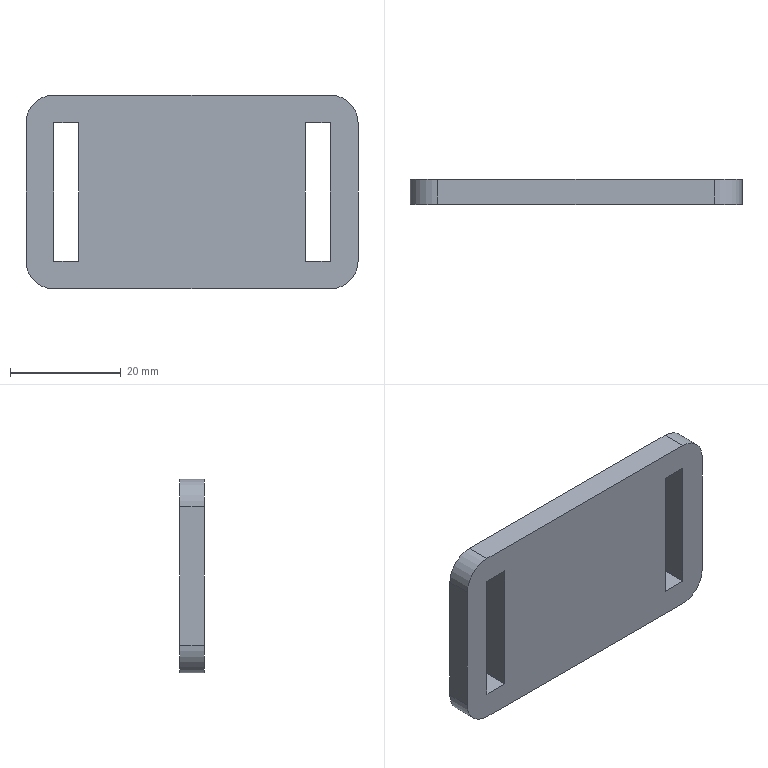Part | SolidWorks | features FlatPattern 1, SMBaseFlange 1, SheetMetal 1 | 1 solid | 18 faces | box 60 x 4.5 x 35 mm | volume 8341 mm3 | plane 14 | cylinder 4 | commonest cylinder face diameters 10 x4
STEP:
#1=CARTESIAN_POINT('',(-30.,0.,12.5));
#2=VERTEX_POINT('',#1);
#3=CARTESIAN_POINT('',(-25.,0.,17.5));
#4=VERTEX_POINT('',#3);
#5=CARTESIAN_POINT('',(-25.,0.,12.5));
#6=DIRECTION('',(0.,1.,0.));
#7=DIRECTION('',(0.,0.,1.));
#8=AXIS2_PLACEMENT_3D('',#5,#6,#7);
#9=CIRCLE('',#8,5.);
#10=EDGE_CURVE('',#2,#4,#9,.T.);
#11=ORIENTED_EDGE('',*,*,#10,.F.);
#12=CARTESIAN_POINT('',(-30.,-4.5,12.5));
#13=VERTEX_POINT('',#12);
#14=CARTESIAN_POINT('',(-30.,-4.5,12.5));
#15=DIRECTION('',(0.,1.,0.));
#16=VECTOR('',#15,1000.);
#17=LINE('',#14,#16);
#18=EDGE_CURVE('',#13,#2,#17,.T.);
#19=ORIENTED_EDGE('',*,*,#18,.F.);
#20=CARTESIAN_POINT('',(-25.,-4.5,17.5));
#21=VERTEX_POINT('',#20);
#22=CARTESIAN_POINT('',(-25.,-4.5,12.5));
#23=DIRECTION('',(0.,1.,0.));
#24=DIRECTION('',(0.,0.,1.));
#25=AXIS2_PLACEMENT_3D('',#22,#23,#24);
#26=CIRCLE('',#25,5.);
#27=EDGE_CURVE('',#13,#21,#26,.T.);
#28=ORIENTED_EDGE('',*,*,#27,.T.);
#29=CARTESIAN_POINT('',(-25.,-4.5,17.5));
#30=DIRECTION('',(0.,1.,0.));
#31=VECTOR('',#30,1000.);
#32=LINE('',#29,#31);
#33=EDGE_CURVE('',#21,#4,#32,.T.);
#34=ORIENTED_EDGE('',*,*,#33,.T.);
#35=EDGE_LOOP('',(#11,#19,#28,#34));
#36=FACE_OUTER_BOUND('',#35,.T.);
#37=CARTESIAN_POINT('',(-25.,-4.5,12.5));
#38=DIRECTION('',(0.,1.,0.));
#39=DIRECTION('',(0.,0.,1.));
#40=AXIS2_PLACEMENT_3D('',#37,#38,#39);
#41=CYLINDRICAL_SURFACE('',#40,5.);
#42=ADVANCED_FACE('',(#36),#41,.T.);
#43=CARTESIAN_POINT('',(-30.,0.,-12.5));
#44=VERTEX_POINT('',#43);
#45=CARTESIAN_POINT('',(-30.,0.,-12.5));
#46=DIRECTION('',(0.,0.,1.));
#47=VECTOR('',#46,1000.);
#48=LINE('',#45,#47);
#49=EDGE_CURVE('',#44,#2,#48,.T.);
#50=ORIENTED_EDGE('',*,*,#49,.F.);
#51=CARTESIAN_POINT('',(-30.,-4.5,-12.5));
#52=VERTEX_POINT('',#51);
#53=CARTESIAN_POINT('',(-30.,-4.5,-12.5));
#54=DIRECTION('',(0.,1.,0.));
#55=VECTOR('',#54,1000.);
#56=LINE('',#53,#55);
#57=EDGE_CURVE('',#52,#44,#56,.T.);
#58=ORIENTED_EDGE('',*,*,#57,.F.);
#59=CARTESIAN_POINT('',(-30.,-4.5,-12.5));
#60=DIRECTION('',(0.,0.,1.));
#61=VECTOR('',#60,1000.);
#62=LINE('',#59,#61);
#63=EDGE_CURVE('',#52,#13,#62,.T.);
#64=ORIENTED_EDGE('',*,*,#63,.T.);
#65=ORIENTED_EDGE('',*,*,#18,.T.);
#66=EDGE_LOOP('',(#50,#58,#64,#65));
#67=FACE_OUTER_BOUND('',#66,.T.);
#68=CARTESIAN_POINT('',(-30.,-4.5,-12.5));
#69=DIRECTION('',(-1.,0.,0.));
#70=DIRECTION('',(0.,0.,1.));
#71=AXIS2_PLACEMENT_3D('',#68,#69,#70);
#72=PLANE('',#71);
#73=ADVANCED_FACE('',(#67),#72,.T.);
#74=CARTESIAN_POINT('',(-25.,0.,-17.5));
#75=VERTEX_POINT('',#74);
#76=CARTESIAN_POINT('',(-25.,0.,-12.5));
#77=DIRECTION('',(0.,1.,0.));
#78=DIRECTION('',(0.,0.,1.));
#79=AXIS2_PLACEMENT_3D('',#76,#77,#78);
#80=CIRCLE('',#79,5.);
#81=EDGE_CURVE('',#75,#44,#80,.T.);
#82=ORIENTED_EDGE('',*,*,#81,.F.);
#83=CARTESIAN_POINT('',(-25.,-4.5,-17.5));
#84=VERTEX_POINT('',#83);
#85=CARTESIAN_POINT('',(-25.,-4.5,-17.5));
#86=DIRECTION('',(0.,1.,0.));
#87=VECTOR('',#86,1000.);
#88=LINE('',#85,#87);
#89=EDGE_CURVE('',#84,#75,#88,.T.);
#90=ORIENTED_EDGE('',*,*,#89,.F.);
#91=CARTESIAN_POINT('',(-25.,-4.5,-12.5));
#92=DIRECTION('',(0.,1.,0.));
#93=DIRECTION('',(0.,0.,1.));
#94=AXIS2_PLACEMENT_3D('',#91,#92,#93);
#95=CIRCLE('',#94,5.);
#96=EDGE_CURVE('',#84,#52,#95,.T.);
#97=ORIENTED_EDGE('',*,*,#96,.T.);
#98=ORIENTED_EDGE('',*,*,#57,.T.);
#99=EDGE_LOOP('',(#82,#90,#97,#98));
#100=FACE_OUTER_BOUND('',#99,.T.);
#101=CARTESIAN_POINT('',(-25.,-4.5,-12.5));
#102=DIRECTION('',(0.,1.,0.));
#103=DIRECTION('',(0.,0.,1.));
#104=AXIS2_PLACEMENT_3D('',#101,#102,#103);
#105=CYLINDRICAL_SURFACE('',#104,5.);
#106=ADVANCED_FACE('',(#100),#105,.T.);
#107=CARTESIAN_POINT('',(25.,0.,-17.5));
#108=VERTEX_POINT('',#107);
#109=CARTESIAN_POINT('',(-25.,0.,-17.5));
#110=DIRECTION('',(-1.,0.,0.));
#111=VECTOR('',#110,1000.);
#112=LINE('',#109,#111);
#113=EDGE_CURVE('',#108,#75,#112,.T.);
#114=ORIENTED_EDGE('',*,*,#113,.F.);
#115=CARTESIAN_POINT('',(25.,-4.5,-17.5));
#116=VERTEX_POINT('',#115);
#117=CARTESIAN_POINT('',(25.,-4.5,-17.5));
#118=DIRECTION('',(0.,1.,0.));
#119=VECTOR('',#118,1000.);
#120=LINE('',#117,#119);
#121=EDGE_CURVE('',#116,#108,#120,.T.);
#122=ORIENTED_EDGE('',*,*,#121,.F.);
#123=CARTESIAN_POINT('',(-25.,-4.5,-17.5));
#124=DIRECTION('',(-1.,0.,0.));
#125=VECTOR('',#124,1000.);
#126=LINE('',#123,#125);
#127=EDGE_CURVE('',#116,#84,#126,.T.);
#128=ORIENTED_EDGE('',*,*,#127,.T.);
#129=ORIENTED_EDGE('',*,*,#89,.T.);
#130=EDGE_LOOP('',(#114,#122,#128,#129));
#131=FACE_OUTER_BOUND('',#130,.T.);
#132=CARTESIAN_POINT('',(-25.,-4.5,-17.5));
#133=DIRECTION('',(0.,0.,-1.));
#134=DIRECTION('',(-1.,0.,0.));
#135=AXIS2_PLACEMENT_3D('',#132,#133,#134);
#136=PLANE('',#135);
#137=ADVANCED_FACE('',(#131),#136,.T.);
#138=CARTESIAN_POINT('',(30.,0.,-12.5));
#139=VERTEX_POINT('',#138);
#140=CARTESIAN_POINT('',(25.,0.,-12.5));
#141=DIRECTION('',(0.,1.,0.));
#142=DIRECTION('',(0.,0.,-1.));
#143=AXIS2_PLACEMENT_3D('',#140,#141,#142);
#144=CIRCLE('',#143,5.);
#145=EDGE_CURVE('',#139,#108,#144,.T.);
#146=ORIENTED_EDGE('',*,*,#145,.F.);
#147=CARTESIAN_POINT('',(30.,-4.5,-12.5));
#148=VERTEX_POINT('',#147);
#149=CARTESIAN_POINT('',(30.,-4.5,-12.5));
#150=DIRECTION('',(0.,1.,0.));
#151=VECTOR('',#150,1000.);
#152=LINE('',#149,#151);
#153=EDGE_CURVE('',#148,#139,#152,.T.);
#154=ORIENTED_EDGE('',*,*,#153,.F.);
#155=CARTESIAN_POINT('',(25.,-4.5,-12.5));
#156=DIRECTION('',(0.,1.,0.));
#157=DIRECTION('',(0.,0.,-1.));
#158=AXIS2_PLACEMENT_3D('',#155,#156,#157);
#159=CIRCLE('',#158,5.);
#160=EDGE_CURVE('',#148,#116,#159,.T.);
#161=ORIENTED_EDGE('',*,*,#160,.T.);
#162=ORIENTED_EDGE('',*,*,#121,.T.);
#163=EDGE_LOOP('',(#146,#154,#161,#162));
#164=FACE_OUTER_BOUND('',#163,.T.);
#165=CARTESIAN_POINT('',(25.,-4.5,-12.5));
#166=DIRECTION('',(0.,1.,0.));
#167=DIRECTION('',(0.,0.,1.));
#168=AXIS2_PLACEMENT_3D('',#165,#166,#167);
#169=CYLINDRICAL_SURFACE('',#168,5.);
#170=ADVANCED_FACE('',(#164),#169,.T.);
#171=CARTESIAN_POINT('',(30.,0.,12.5));
#172=VERTEX_POINT('',#171);
#173=CARTESIAN_POINT('',(30.,0.,-12.5));
#174=DIRECTION('',(0.,0.,-1.));
#175=VECTOR('',#174,1000.);
#176=LINE('',#173,#175);
#177=EDGE_CURVE('',#172,#139,#176,.T.);
#178=ORIENTED_EDGE('',*,*,#177,.F.);
#179=CARTESIAN_POINT('',(30.,-4.5,12.5));
#180=VERTEX_POINT('',#179);
#181=CARTESIAN_POINT('',(30.,-4.5,12.5));
#182=DIRECTION('',(0.,1.,0.));
#183=VECTOR('',#182,1000.);
#184=LINE('',#181,#183);
#185=EDGE_CURVE('',#180,#172,#184,.T.);
#186=ORIENTED_EDGE('',*,*,#185,.F.);
#187=CARTESIAN_POINT('',(30.,-4.5,-12.5));
#188=DIRECTION('',(0.,0.,-1.));
#189=VECTOR('',#188,1000.);
#190=LINE('',#187,#189);
#191=EDGE_CURVE('',#180,#148,#190,.T.);
#192=ORIENTED_EDGE('',*,*,#191,.T.);
#193=ORIENTED_EDGE('',*,*,#153,.T.);
#194=EDGE_LOOP('',(#178,#186,#192,#193));
#195=FACE_OUTER_BOUND('',#194,.T.);
#196=CARTESIAN_POINT('',(30.,-4.5,-12.5));
#197=DIRECTION('',(1.,0.,0.));
#198=DIRECTION('',(0.,0.,-1.));
#199=AXIS2_PLACEMENT_3D('',#196,#197,#198);
#200=PLANE('',#199);
#201=ADVANCED_FACE('',(#195),#200,.T.);
#202=CARTESIAN_POINT('',(25.,0.,17.5));
#203=VERTEX_POINT('',#202);
#204=CARTESIAN_POINT('',(25.,0.,12.5));
#205=DIRECTION('',(0.,1.,0.));
#206=DIRECTION('',(0.,0.,1.));
#207=AXIS2_PLACEMENT_3D('',#204,#205,#206);
#208=CIRCLE('',#207,5.);
#209=EDGE_CURVE('',#203,#172,#208,.T.);
#210=ORIENTED_EDGE('',*,*,#209,.F.);
#211=CARTESIAN_POINT('',(25.,-4.5,17.5));
#212=VERTEX_POINT('',#211);
#213=CARTESIAN_POINT('',(25.,-4.5,17.5));
#214=DIRECTION('',(0.,1.,0.));
#215=VECTOR('',#214,1000.);
#216=LINE('',#213,#215);
#217=EDGE_CURVE('',#212,#203,#216,.T.);
#218=ORIENTED_EDGE('',*,*,#217,.F.);
#219=CARTESIAN_POINT('',(25.,-4.5,12.5));
#220=DIRECTION('',(0.,1.,0.));
#221=DIRECTION('',(0.,0.,1.));
#222=AXIS2_PLACEMENT_3D('',#219,#220,#221);
#223=CIRCLE('',#222,5.);
#224=EDGE_CURVE('',#212,#180,#223,.T.);
#225=ORIENTED_EDGE('',*,*,#224,.T.);
#226=ORIENTED_EDGE('',*,*,#185,.T.);
#227=EDGE_LOOP('',(#210,#218,#225,#226));
#228=FACE_OUTER_BOUND('',#227,.T.);
#229=CARTESIAN_POINT('',(25.,-4.5,12.5));
#230=DIRECTION('',(0.,1.,0.));
#231=DIRECTION('',(0.,0.,1.));
#232=AXIS2_PLACEMENT_3D('',#229,#230,#231);
#233=CYLINDRICAL_SURFACE('',#232,5.);
#234=ADVANCED_FACE('',(#228),#233,.T.);
#235=CARTESIAN_POINT('',(-25.,0.,17.5));
#236=DIRECTION('',(1.,0.,0.));
#237=VECTOR('',#236,1000.);
#238=LINE('',#235,#237);
#239=EDGE_CURVE('',#4,#203,#238,.T.);
#240=ORIENTED_EDGE('',*,*,#239,.F.);
#241=ORIENTED_EDGE('',*,*,#33,.F.);
#242=CARTESIAN_POINT('',(-25.,-4.5,17.5));
#243=DIRECTION('',(1.,0.,0.));
#244=VECTOR('',#243,1000.);
#245=LINE('',#242,#244);
#246=EDGE_CURVE('',#21,#212,#245,.T.);
#247=ORIENTED_EDGE('',*,*,#246,.T.);
#248=ORIENTED_EDGE('',*,*,#217,.T.);
#249=EDGE_LOOP('',(#240,#241,#247,#248));
#250=FACE_OUTER_BOUND('',#249,.T.);
#251=CARTESIAN_POINT('',(-25.,-4.5,17.5));
#252=DIRECTION('',(0.,0.,1.));
#253=DIRECTION('',(1.,0.,0.));
#254=AXIS2_PLACEMENT_3D('',#251,#252,#253);
#255=PLANE('',#254);
#256=ADVANCED_FACE('',(#250),#255,.T.);
#257=CARTESIAN_POINT('',(25.,-4.5,12.5));
#258=VERTEX_POINT('',#257);
#259=CARTESIAN_POINT('',(25.,-4.5,-12.5));
#260=VERTEX_POINT('',#259);
#261=CARTESIAN_POINT('',(25.,-4.5,-12.5));
#262=DIRECTION('',(0.,0.,-1.));
#263=VECTOR('',#262,1000.);
#264=LINE('',#261,#263);
#265=EDGE_CURVE('',#258,#260,#264,.T.);
#266=ORIENTED_EDGE('',*,*,#265,.T.);
#267=CARTESIAN_POINT('',(20.5,-4.5,-12.5));
#268=VERTEX_POINT('',#267);
#269=CARTESIAN_POINT('',(25.,-4.5,-12.5));
#270=DIRECTION('',(-1.,0.,0.));
#271=VECTOR('',#270,1000.);
#272=LINE('',#269,#271);
#273=EDGE_CURVE('',#260,#268,#272,.T.);
#274=ORIENTED_EDGE('',*,*,#273,.T.);
#275=CARTESIAN_POINT('',(20.5,-4.5,12.5));
#276=VERTEX_POINT('',#275);
#277=CARTESIAN_POINT('',(20.5,-4.5,-12.5));
#278=DIRECTION('',(0.,0.,1.));
#279=VECTOR('',#278,1000.);
#280=LINE('',#277,#279);
#281=EDGE_CURVE('',#268,#276,#280,.T.);
#282=ORIENTED_EDGE('',*,*,#281,.T.);
#283=CARTESIAN_POINT('',(25.,-4.5,12.5));
#284=DIRECTION('',(1.,0.,0.));
#285=VECTOR('',#284,1000.);
#286=LINE('',#283,#285);
#287=EDGE_CURVE('',#276,#258,#286,.T.);
#288=ORIENTED_EDGE('',*,*,#287,.T.);
#289=EDGE_LOOP('',(#266,#274,#282,#288));
#290=FACE_BOUND('',#289,.T.);
#291=CARTESIAN_POINT('',(-20.5,-4.5,-12.5));
#292=VERTEX_POINT('',#291);
#293=CARTESIAN_POINT('',(-25.,-4.5,-12.5));
#294=VERTEX_POINT('',#293);
#295=CARTESIAN_POINT('',(-25.,-4.5,-12.5));
#296=DIRECTION('',(-1.,0.,0.));
#297=VECTOR('',#296,1000.);
#298=LINE('',#295,#297);
#299=EDGE_CURVE('',#292,#294,#298,.T.);
#300=ORIENTED_EDGE('',*,*,#299,.T.);
#301=CARTESIAN_POINT('',(-25.,-4.5,12.5));
#302=VERTEX_POINT('',#301);
#303=CARTESIAN_POINT('',(-25.,-4.5,-12.5));
#304=DIRECTION('',(0.,0.,1.));
#305=VECTOR('',#304,1000.);
#306=LINE('',#303,#305);
#307=EDGE_CURVE('',#294,#302,#306,.T.);
#308=ORIENTED_EDGE('',*,*,#307,.T.);
#309=CARTESIAN_POINT('',(-20.5,-4.5,12.5));
#310=VERTEX_POINT('',#309);
#311=CARTESIAN_POINT('',(-25.,-4.5,12.5));
#312=DIRECTION('',(1.,0.,0.));
#313=VECTOR('',#312,1000.);
#314=LINE('',#311,#313);
#315=EDGE_CURVE('',#302,#310,#314,.T.);
#316=ORIENTED_EDGE('',*,*,#315,.T.);
#317=CARTESIAN_POINT('',(-20.5,-4.5,-12.5));
#318=DIRECTION('',(0.,0.,-1.));
#319=VECTOR('',#318,1000.);
#320=LINE('',#317,#319);
#321=EDGE_CURVE('',#310,#292,#320,.T.);
#322=ORIENTED_EDGE('',*,*,#321,.T.);
#323=EDGE_LOOP('',(#300,#308,#316,#322));
#324=FACE_BOUND('',#323,.T.);
#325=ORIENTED_EDGE('',*,*,#27,.F.);
#326=ORIENTED_EDGE('',*,*,#63,.F.);
#327=ORIENTED_EDGE('',*,*,#96,.F.);
#328=ORIENTED_EDGE('',*,*,#127,.F.);
#329=ORIENTED_EDGE('',*,*,#160,.F.);
#330=ORIENTED_EDGE('',*,*,#191,.F.);
#331=ORIENTED_EDGE('',*,*,#224,.F.);
#332=ORIENTED_EDGE('',*,*,#246,.F.);
#333=EDGE_LOOP('',(#325,#326,#327,#328,#329,#330,#331,#332));
#334=FACE_OUTER_BOUND('',#333,.T.);
#335=CARTESIAN_POINT('',(-25.,-4.5,12.5));
#336=DIRECTION('',(0.,1.,0.));
#337=DIRECTION('',(0.,0.,1.));
#338=AXIS2_PLACEMENT_3D('',#335,#336,#337);
#339=PLANE('',#338);
#340=ADVANCED_FACE('',(#290,#324,#334),#339,.F.);
#341=CARTESIAN_POINT('',(25.,0.,-12.5));
#342=VERTEX_POINT('',#341);
#343=CARTESIAN_POINT('',(20.5,0.,-12.5));
#344=VERTEX_POINT('',#343);
#345=CARTESIAN_POINT('',(25.,0.,-12.5));
#346=DIRECTION('',(-1.,0.,0.));
#347=VECTOR('',#346,1000.);
#348=LINE('',#345,#347);
#349=EDGE_CURVE('',#342,#344,#348,.T.);
#350=ORIENTED_EDGE('',*,*,#349,.F.);
#351=CARTESIAN_POINT('',(25.,0.,12.5));
#352=VERTEX_POINT('',#351);
#353=CARTESIAN_POINT('',(25.,0.,-12.5));
#354=DIRECTION('',(0.,0.,-1.));
#355=VECTOR('',#354,1000.);
#356=LINE('',#353,#355);
#357=EDGE_CURVE('',#352,#342,#356,.T.);
#358=ORIENTED_EDGE('',*,*,#357,.F.);
#359=CARTESIAN_POINT('',(20.5,0.,12.5));
#360=VERTEX_POINT('',#359);
#361=CARTESIAN_POINT('',(25.,0.,12.5));
#362=DIRECTION('',(1.,0.,0.));
#363=VECTOR('',#362,1000.);
#364=LINE('',#361,#363);
#365=EDGE_CURVE('',#360,#352,#364,.T.);
#366=ORIENTED_EDGE('',*,*,#365,.F.);
#367=CARTESIAN_POINT('',(20.5,0.,-12.5));
#368=DIRECTION('',(0.,0.,1.));
#369=VECTOR('',#368,1000.);
#370=LINE('',#367,#369);
#371=EDGE_CURVE('',#344,#360,#370,.T.);
#372=ORIENTED_EDGE('',*,*,#371,.F.);
#373=EDGE_LOOP('',(#350,#358,#366,#372));
#374=FACE_BOUND('',#373,.T.);
#375=CARTESIAN_POINT('',(-25.,0.,-12.5));
#376=VERTEX_POINT('',#375);
#377=CARTESIAN_POINT('',(-25.,0.,12.5));
#378=VERTEX_POINT('',#377);
#379=CARTESIAN_POINT('',(-25.,0.,-12.5));
#380=DIRECTION('',(0.,0.,1.));
#381=VECTOR('',#380,1000.);
#382=LINE('',#379,#381);
#383=EDGE_CURVE('',#376,#378,#382,.T.);
#384=ORIENTED_EDGE('',*,*,#383,.F.);
#385=CARTESIAN_POINT('',(-20.5,0.,-12.5));
#386=VERTEX_POINT('',#385);
#387=CARTESIAN_POINT('',(-25.,0.,-12.5));
#388=DIRECTION('',(-1.,0.,0.));
#389=VECTOR('',#388,1000.);
#390=LINE('',#387,#389);
#391=EDGE_CURVE('',#386,#376,#390,.T.);
#392=ORIENTED_EDGE('',*,*,#391,.F.);
#393=CARTESIAN_POINT('',(-20.5,0.,12.5));
#394=VERTEX_POINT('',#393);
#395=CARTESIAN_POINT('',(-20.5,0.,-12.5));
#396=DIRECTION('',(0.,0.,-1.));
#397=VECTOR('',#396,1000.);
#398=LINE('',#395,#397);
#399=EDGE_CURVE('',#394,#386,#398,.T.);
#400=ORIENTED_EDGE('',*,*,#399,.F.);
#401=CARTESIAN_POINT('',(-25.,0.,12.5));
#402=DIRECTION('',(1.,0.,0.));
#403=VECTOR('',#402,1000.);
#404=LINE('',#401,#403);
#405=EDGE_CURVE('',#378,#394,#404,.T.);
#406=ORIENTED_EDGE('',*,*,#405,.F.);
#407=EDGE_LOOP('',(#384,#392,#400,#406));
#408=FACE_BOUND('',#407,.T.);
#409=ORIENTED_EDGE('',*,*,#10,.T.);
#410=ORIENTED_EDGE('',*,*,#239,.T.);
#411=ORIENTED_EDGE('',*,*,#209,.T.);
#412=ORIENTED_EDGE('',*,*,#177,.T.);
#413=ORIENTED_EDGE('',*,*,#145,.T.);
#414=ORIENTED_EDGE('',*,*,#113,.T.);
#415=ORIENTED_EDGE('',*,*,#81,.T.);
#416=ORIENTED_EDGE('',*,*,#49,.T.);
#417=EDGE_LOOP('',(#409,#410,#411,#412,#413,#414,#415,#416));
#418=FACE_OUTER_BOUND('',#417,.T.);
#419=CARTESIAN_POINT('',(-25.,0.,12.5));
#420=DIRECTION('',(0.,1.,0.));
#421=DIRECTION('',(0.,0.,1.));
#422=AXIS2_PLACEMENT_3D('',#419,#420,#421);
#423=PLANE('',#422);
#424=ADVANCED_FACE('',(#374,#408,#418),#423,.T.);
#425=ORIENTED_EDGE('',*,*,#383,.T.);
#426=CARTESIAN_POINT('',(-25.,-4.5,12.5));
#427=DIRECTION('',(0.,1.,0.));
#428=VECTOR('',#427,1000.);
#429=LINE('',#426,#428);
#430=EDGE_CURVE('',#302,#378,#429,.T.);
#431=ORIENTED_EDGE('',*,*,#430,.F.);
#432=ORIENTED_EDGE('',*,*,#307,.F.);
#433=CARTESIAN_POINT('',(-25.,-4.5,-12.5));
#434=DIRECTION('',(0.,1.,0.));
#435=VECTOR('',#434,1000.);
#436=LINE('',#433,#435);
#437=EDGE_CURVE('',#294,#376,#436,.T.);
#438=ORIENTED_EDGE('',*,*,#437,.T.);
#439=EDGE_LOOP('',(#425,#431,#432,#438));
#440=FACE_OUTER_BOUND('',#439,.T.);
#441=CARTESIAN_POINT('',(-25.,-4.5,-12.5));
#442=DIRECTION('',(-1.,0.,0.));
#443=DIRECTION('',(0.,0.,1.));
#444=AXIS2_PLACEMENT_3D('',#441,#442,#443);
#445=PLANE('',#444);
#446=ADVANCED_FACE('',(#440),#445,.F.);
#447=ORIENTED_EDGE('',*,*,#391,.T.);
#448=ORIENTED_EDGE('',*,*,#437,.F.);
#449=ORIENTED_EDGE('',*,*,#299,.F.);
#450=CARTESIAN_POINT('',(-20.5,-4.5,-12.5));
#451=DIRECTION('',(0.,1.,0.));
#452=VECTOR('',#451,1000.);
#453=LINE('',#450,#452);
#454=EDGE_CURVE('',#292,#386,#453,.T.);
#455=ORIENTED_EDGE('',*,*,#454,.T.);
#456=EDGE_LOOP('',(#447,#448,#449,#455));
#457=FACE_OUTER_BOUND('',#456,.T.);
#458=CARTESIAN_POINT('',(-25.,-4.5,-12.5));
#459=DIRECTION('',(0.,0.,-1.));
#460=DIRECTION('',(-1.,0.,0.));
#461=AXIS2_PLACEMENT_3D('',#458,#459,#460);
#462=PLANE('',#461);
#463=ADVANCED_FACE('',(#457),#462,.F.);
#464=ORIENTED_EDGE('',*,*,#399,.T.);
#465=ORIENTED_EDGE('',*,*,#454,.F.);
#466=ORIENTED_EDGE('',*,*,#321,.F.);
#467=CARTESIAN_POINT('',(-20.5,-4.5,12.5));
#468=DIRECTION('',(0.,1.,0.));
#469=VECTOR('',#468,1000.);
#470=LINE('',#467,#469);
#471=EDGE_CURVE('',#310,#394,#470,.T.);
#472=ORIENTED_EDGE('',*,*,#471,.T.);
#473=EDGE_LOOP('',(#464,#465,#466,#472));
#474=FACE_OUTER_BOUND('',#473,.T.);
#475=CARTESIAN_POINT('',(-20.5,-4.5,-12.5));
#476=DIRECTION('',(1.,0.,0.));
#477=DIRECTION('',(0.,0.,-1.));
#478=AXIS2_PLACEMENT_3D('',#475,#476,#477);
#479=PLANE('',#478);
#480=ADVANCED_FACE('',(#474),#479,.F.);
#481=ORIENTED_EDGE('',*,*,#405,.T.);
#482=ORIENTED_EDGE('',*,*,#471,.F.);
#483=ORIENTED_EDGE('',*,*,#315,.F.);
#484=ORIENTED_EDGE('',*,*,#430,.T.);
#485=EDGE_LOOP('',(#481,#482,#483,#484));
#486=FACE_OUTER_BOUND('',#485,.T.);
#487=CARTESIAN_POINT('',(-25.,-4.5,12.5));
#488=DIRECTION('',(0.,0.,1.));
#489=DIRECTION('',(1.,0.,0.));
#490=AXIS2_PLACEMENT_3D('',#487,#488,#489);
#491=PLANE('',#490);
#492=ADVANCED_FACE('',(#486),#491,.F.);
#493=ORIENTED_EDGE('',*,*,#349,.T.);
#494=CARTESIAN_POINT('',(20.5,-4.5,-12.5));
#495=DIRECTION('',(0.,1.,0.));
#496=VECTOR('',#495,1000.);
#497=LINE('',#494,#496);
#498=EDGE_CURVE('',#268,#344,#497,.T.);
#499=ORIENTED_EDGE('',*,*,#498,.F.);
#500=ORIENTED_EDGE('',*,*,#273,.F.);
#501=CARTESIAN_POINT('',(25.,-4.5,-12.5));
#502=DIRECTION('',(0.,1.,0.));
#503=VECTOR('',#502,1000.);
#504=LINE('',#501,#503);
#505=EDGE_CURVE('',#260,#342,#504,.T.);
#506=ORIENTED_EDGE('',*,*,#505,.T.);
#507=EDGE_LOOP('',(#493,#499,#500,#506));
#508=FACE_OUTER_BOUND('',#507,.T.);
#509=CARTESIAN_POINT('',(25.,-4.5,-12.5));
#510=DIRECTION('',(0.,0.,-1.));
#511=DIRECTION('',(-1.,0.,0.));
#512=AXIS2_PLACEMENT_3D('',#509,#510,#511);
#513=PLANE('',#512);
#514=ADVANCED_FACE('',(#508),#513,.F.);
#515=ORIENTED_EDGE('',*,*,#357,.T.);
#516=ORIENTED_EDGE('',*,*,#505,.F.);
#517=ORIENTED_EDGE('',*,*,#265,.F.);
#518=CARTESIAN_POINT('',(25.,-4.5,12.5));
#519=DIRECTION('',(0.,1.,0.));
#520=VECTOR('',#519,1000.);
#521=LINE('',#518,#520);
#522=EDGE_CURVE('',#258,#352,#521,.T.);
#523=ORIENTED_EDGE('',*,*,#522,.T.);
#524=EDGE_LOOP('',(#515,#516,#517,#523));
#525=FACE_OUTER_BOUND('',#524,.T.);
#526=CARTESIAN_POINT('',(25.,-4.5,-12.5));
#527=DIRECTION('',(1.,0.,0.));
#528=DIRECTION('',(0.,0.,-1.));
#529=AXIS2_PLACEMENT_3D('',#526,#527,#528);
#530=PLANE('',#529);
#531=ADVANCED_FACE('',(#525),#530,.F.);
#532=ORIENTED_EDGE('',*,*,#365,.T.);
#533=ORIENTED_EDGE('',*,*,#522,.F.);
#534=ORIENTED_EDGE('',*,*,#287,.F.);
#535=CARTESIAN_POINT('',(20.5,-4.5,12.5));
#536=DIRECTION('',(0.,1.,0.));
#537=VECTOR('',#536,1000.);
#538=LINE('',#535,#537);
#539=EDGE_CURVE('',#276,#360,#538,.T.);
#540=ORIENTED_EDGE('',*,*,#539,.T.);
#541=EDGE_LOOP('',(#532,#533,#534,#540));
#542=FACE_OUTER_BOUND('',#541,.T.);
#543=CARTESIAN_POINT('',(25.,-4.5,12.5));
#544=DIRECTION('',(0.,0.,1.));
#545=DIRECTION('',(1.,0.,0.));
#546=AXIS2_PLACEMENT_3D('',#543,#544,#545);
#547=PLANE('',#546);
#548=ADVANCED_FACE('',(#542),#547,.F.);
#549=ORIENTED_EDGE('',*,*,#371,.T.);
#550=ORIENTED_EDGE('',*,*,#539,.F.);
#551=ORIENTED_EDGE('',*,*,#281,.F.);
#552=ORIENTED_EDGE('',*,*,#498,.T.);
#553=EDGE_LOOP('',(#549,#550,#551,#552));
#554=FACE_OUTER_BOUND('',#553,.T.);
#555=CARTESIAN_POINT('',(20.5,-4.5,-12.5));
#556=DIRECTION('',(-1.,0.,0.));
#557=DIRECTION('',(0.,0.,1.));
#558=AXIS2_PLACEMENT_3D('',#555,#556,#557);
#559=PLANE('',#558);
#560=ADVANCED_FACE('',(#554),#559,.F.);
#561=CLOSED_SHELL('',(#42,#73,#106,#137,#170,#201,#234,#256,#340,#424,#446,#463,#480,#492,#514,#531,#548,#560));
#562=MANIFOLD_SOLID_BREP('',#561);
#563=CARTESIAN_POINT('',(0.,0.,0.));
#564=DIRECTION('',(0.,0.,1.));
#565=DIRECTION('',(1.,0.,0.));
#566=AXIS2_PLACEMENT_3D('',#563,#564,#565);
#567=(LENGTH_UNIT()NAMED_UNIT(*)SI_UNIT(.MILLI.,.METRE.));
#568=UNCERTAINTY_MEASURE_WITH_UNIT(LENGTH_MEASURE(0.00001),#567,'','');
#569=(NAMED_UNIT(*)PLANE_ANGLE_UNIT()SI_UNIT($,.RADIAN.));
#570=(NAMED_UNIT(*)SI_UNIT($,.STERADIAN.)SOLID_ANGLE_UNIT());
#571=(GEOMETRIC_REPRESENTATION_CONTEXT(3)GLOBAL_UNCERTAINTY_ASSIGNED_CONTEXT((#568))GLOBAL_UNIT_ASSIGNED_CONTEXT((#567,#569,#570))REPRESENTATION_CONTEXT('',''));
#572=ADVANCED_BREP_SHAPE_REPRESENTATION('',(#562,#566),#571);